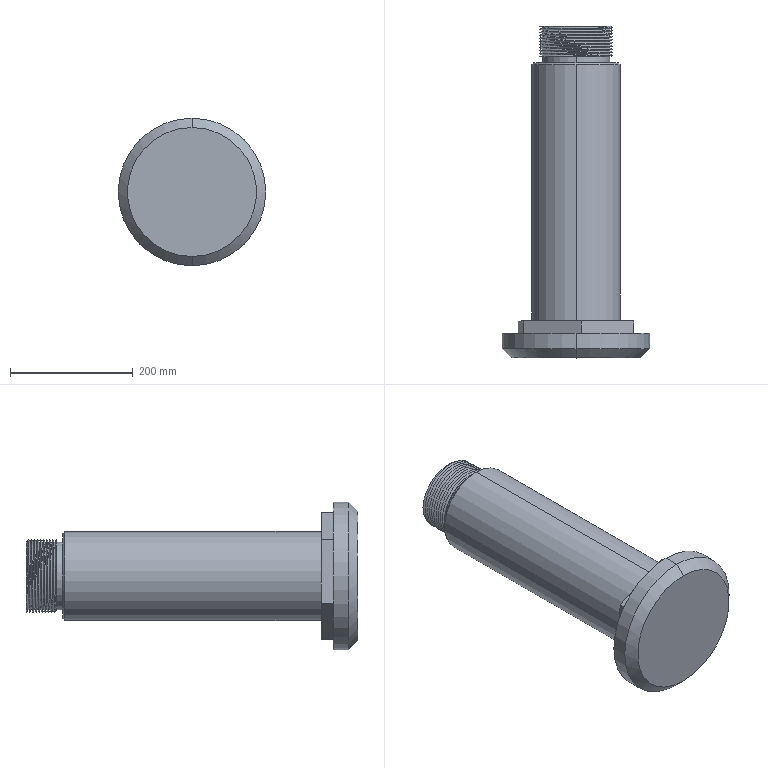Part | SolidWorks | features ICE 4, Chamfer 2, Extrusion 1, Helix 1, SweepCut 1 | 1 solid | 24 faces | box 240 x 540 x 240 mm | volume 9830970 mm3 | plane 12 | cylinder 6 | cone 4 | spline 2 | commonest cylinder face diameters 110 x2 145 x2 240 x2